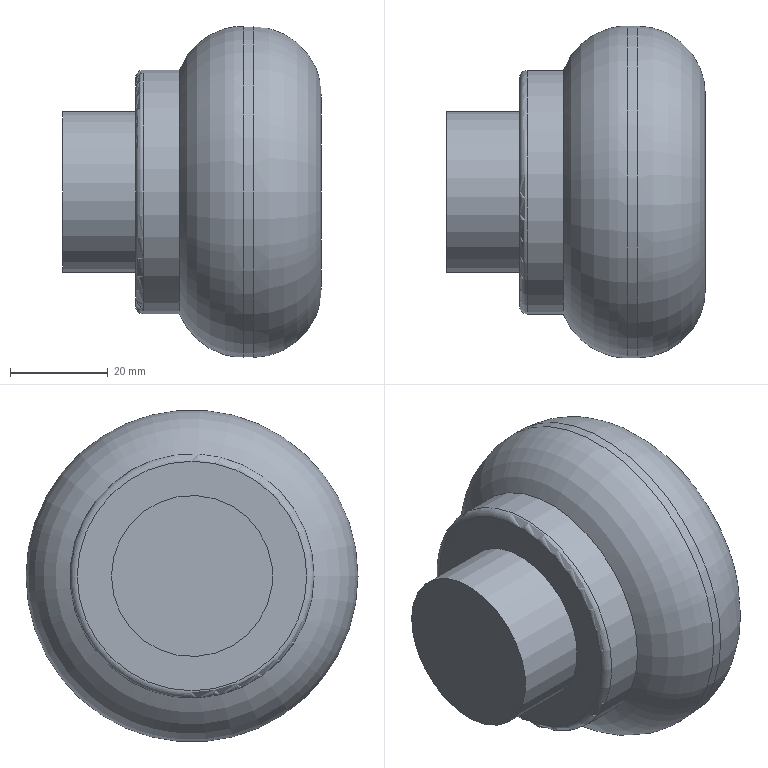Part | STEP file | CMT7E v7 | 1 solid | 11 faces | box 53 x 68 x 68 mm | volume 121265 mm3 | plane 4 | cylinder 4 | torus 3 | commonest cylinder face diameters 6 x1 33 x1 50 x1 68 x1
STEP:
#1=CARTESIAN_POINT('',(0.,0.,0.));
#2=DIRECTION('',(0.,0.,1.));
#3=DIRECTION('',(1.,0.,0.));
#4=AXIS2_PLACEMENT_3D('',#1,#2,#3);
#5=CARTESIAN_POINT('',(95.,16.49,190.));
#6=VERTEX_POINT('',#5);
#7=CARTESIAN_POINT('',(95.,-0.01,190.));
#8=DIRECTION('',(1.,0.,0.));
#9=DIRECTION('',(0.,1.,0.));
#10=AXIS2_PLACEMENT_3D('',#7,#8,#9);
#11=CIRCLE('',#10,16.5);
#12=CARTESIAN_POINT('',(95.,-0.01,190.));
#13=DIRECTION('',(1.,0.,0.));
#14=DIRECTION('',(0.,1.,0.));
#15=AXIS2_PLACEMENT_3D('',#12,#13,#14);
#16=PLANE('',#15);
#17=CARTESIAN_POINT('',(0.,0.));
#18=DIRECTION('',(1.,0.));
#19=AXIS2_PLACEMENT_2D('',#17,#18);
#20=CIRCLE('',#19,16.5);
#21=(GEOMETRIC_REPRESENTATION_CONTEXT(2)PARAMETRIC_REPRESENTATION_CONTEXT()REPRESENTATION_CONTEXT('',''));
#22=DEFINITIONAL_REPRESENTATION('',(#20),#21);
#23=PCURVE('',#16,#22);
#24=CARTESIAN_POINT('',(95.,-0.01,190.));
#25=DIRECTION('',(1.,0.,0.));
#26=DIRECTION('',(0.,1.,0.));
#27=AXIS2_PLACEMENT_3D('',#24,#25,#26);
#28=CYLINDRICAL_SURFACE('',#27,16.5);
#29=CARTESIAN_POINT('',(0.,0.));
#30=DIRECTION('',(1.,0.));
#31=VECTOR('',#30,1.);
#32=LINE('',#29,#31);
#33=(GEOMETRIC_REPRESENTATION_CONTEXT(2)PARAMETRIC_REPRESENTATION_CONTEXT()REPRESENTATION_CONTEXT('',''));
#34=DEFINITIONAL_REPRESENTATION('',(#32),#33);
#35=PCURVE('',#28,#34);
#36=SURFACE_CURVE('',#11,(#23,#35),.PCURVE_S1.);
#37=EDGE_CURVE('',#6,#6,#36,.T.);
#38=ORIENTED_EDGE('',*,*,#37,.F.);
#39=EDGE_LOOP('',(#38));
#40=FACE_BOUND('',#39,.T.);
#41=ADVANCED_FACE('',(#40),#16,.F.);
#42=ORIENTED_EDGE('',*,*,#37,.T.);
#43=CARTESIAN_POINT('',(110.,16.49,190.));
#44=VERTEX_POINT('',#43);
#45=CARTESIAN_POINT('',(95.,16.49,190.));
#46=CARTESIAN_POINT('',(110.,16.49,190.));
#47=B_SPLINE_CURVE_WITH_KNOTS('',1,(#45,#46),.UNSPECIFIED.,.F.,.F.,(2,2),(0.,15.),.PIECEWISE_BEZIER_KNOTS.);
#48=CARTESIAN_POINT('',(6.283,0.));
#49=DIRECTION('',(0.,1.));
#50=VECTOR('',#49,1.);
#51=LINE('',#48,#50);
#52=(GEOMETRIC_REPRESENTATION_CONTEXT(2)PARAMETRIC_REPRESENTATION_CONTEXT()REPRESENTATION_CONTEXT('',''));
#53=DEFINITIONAL_REPRESENTATION('',(#51),#52);
#54=PCURVE('',#28,#53);
#55=CARTESIAN_POINT('',(0.,0.));
#56=DIRECTION('',(0.,1.));
#57=VECTOR('',#56,1.);
#58=LINE('',#55,#57);
#59=(GEOMETRIC_REPRESENTATION_CONTEXT(2)PARAMETRIC_REPRESENTATION_CONTEXT()REPRESENTATION_CONTEXT('',''));
#60=DEFINITIONAL_REPRESENTATION('',(#58),#59);
#61=PCURVE('',#28,#60);
#62=SEAM_CURVE('',#47,(#54,#61),.PCURVE_S1.);
#63=EDGE_CURVE('',#6,#44,#62,.T.);
#64=ORIENTED_EDGE('',*,*,#63,.T.);
#65=CARTESIAN_POINT('',(110.,-0.01,190.));
#66=DIRECTION('',(-1.,0.,0.));
#67=DIRECTION('',(0.,1.,0.));
#68=AXIS2_PLACEMENT_3D('',#65,#66,#67);
#69=CIRCLE('',#68,16.5);
#70=CARTESIAN_POINT('',(6.283,15.));
#71=DIRECTION('',(-1.,0.));
#72=VECTOR('',#71,1.);
#73=LINE('',#70,#72);
#74=(GEOMETRIC_REPRESENTATION_CONTEXT(2)PARAMETRIC_REPRESENTATION_CONTEXT()REPRESENTATION_CONTEXT('',''));
#75=DEFINITIONAL_REPRESENTATION('',(#73),#74);
#76=PCURVE('',#28,#75);
#77=CARTESIAN_POINT('',(110.,-0.01,190.));
#78=DIRECTION('',(-1.,0.,0.));
#79=DIRECTION('',(0.,-1.,0.));
#80=AXIS2_PLACEMENT_3D('',#77,#78,#79);
#81=PLANE('',#80);
#82=CARTESIAN_POINT('',(0.,0.));
#83=DIRECTION('',(-1.,0.));
#84=AXIS2_PLACEMENT_2D('',#82,#83);
#85=CIRCLE('',#84,16.5);
#86=(GEOMETRIC_REPRESENTATION_CONTEXT(2)PARAMETRIC_REPRESENTATION_CONTEXT()REPRESENTATION_CONTEXT('',''));
#87=DEFINITIONAL_REPRESENTATION('',(#85),#86);
#88=PCURVE('',#81,#87);
#89=SURFACE_CURVE('',#69,(#76,#88),.PCURVE_S1.);
#90=EDGE_CURVE('',#44,#44,#89,.T.);
#91=ORIENTED_EDGE('',*,*,#90,.T.);
#92=ORIENTED_EDGE('',*,*,#63,.F.);
#93=EDGE_LOOP('',(#42,#64,#91,#92));
#94=FACE_BOUND('',#93,.T.);
#95=ADVANCED_FACE('',(#94),#28,.T.);
#96=CARTESIAN_POINT('',(148.,2.99,190.));
#97=VERTEX_POINT('',#96);
#98=CARTESIAN_POINT('',(148.,-0.01,190.));
#99=DIRECTION('',(-1.,0.,0.));
#100=DIRECTION('',(0.,1.,0.));
#101=AXIS2_PLACEMENT_3D('',#98,#99,#100);
#102=CIRCLE('',#101,3.);
#103=CARTESIAN_POINT('',(148.,-0.01,190.));
#104=DIRECTION('',(1.,0.,0.));
#105=DIRECTION('',(0.,1.,0.));
#106=AXIS2_PLACEMENT_3D('',#103,#104,#105);
#107=PLANE('',#106);
#108=CARTESIAN_POINT('',(3.,0.));
#109=CARTESIAN_POINT('',(3.,-5.196));
#110=CARTESIAN_POINT('',(-1.5,-2.598));
#111=CARTESIAN_POINT('',(-6.,0.));
#112=CARTESIAN_POINT('',(-1.5,2.598));
#113=CARTESIAN_POINT('',(3.,5.196));
#114=CARTESIAN_POINT('',(3.,0.));
#115=(BOUNDED_CURVE()B_SPLINE_CURVE(2,(#108,#109,#110,#111,#112,#113,#114),.UNSPECIFIED.,.T.,.F.)B_SPLINE_CURVE_WITH_KNOTS((1,2,2,2,2,1),(-2.094,0.,2.094,4.189,6.283,8.378),.UNSPECIFIED.)CURVE()GEOMETRIC_REPRESENTATION_ITEM()RATIONAL_B_SPLINE_CURVE((1.,0.5,1.,0.5,1.,0.5,1.))REPRESENTATION_ITEM(''));
#116=(GEOMETRIC_REPRESENTATION_CONTEXT(2)PARAMETRIC_REPRESENTATION_CONTEXT()REPRESENTATION_CONTEXT('',''));
#117=DEFINITIONAL_REPRESENTATION('',(#115),#116);
#118=PCURVE('',#107,#117);
#119=CARTESIAN_POINT('',(148.,-0.01,190.));
#120=DIRECTION('',(-1.,0.,0.));
#121=DIRECTION('',(0.,1.,0.));
#122=AXIS2_PLACEMENT_3D('',#119,#120,#121);
#123=CYLINDRICAL_SURFACE('',#122,3.);
#124=CARTESIAN_POINT('',(0.,0.));
#125=DIRECTION('',(1.,0.));
#126=VECTOR('',#125,1.);
#127=LINE('',#124,#126);
#128=(GEOMETRIC_REPRESENTATION_CONTEXT(2)PARAMETRIC_REPRESENTATION_CONTEXT()REPRESENTATION_CONTEXT('',''));
#129=DEFINITIONAL_REPRESENTATION('',(#127),#128);
#130=PCURVE('',#123,#129);
#131=SURFACE_CURVE('',#102,(#118,#130),.PCURVE_S1.);
#132=EDGE_CURVE('',#97,#97,#131,.T.);
#133=ORIENTED_EDGE('',*,*,#132,.T.);
#134=EDGE_LOOP('',(#133));
#135=FACE_BOUND('',#134,.T.);
#136=CARTESIAN_POINT('',(148.,19.99,190.));
#137=VERTEX_POINT('',#136);
#138=CARTESIAN_POINT('',(148.,-0.01,190.));
#139=DIRECTION('',(-1.,0.,0.));
#140=DIRECTION('',(0.,1.,0.));
#141=AXIS2_PLACEMENT_3D('',#138,#139,#140);
#142=CIRCLE('',#141,20.);
#143=CARTESIAN_POINT('',(20.,0.));
#144=CARTESIAN_POINT('',(20.,-34.641));
#145=CARTESIAN_POINT('',(-10.,-17.321));
#146=CARTESIAN_POINT('',(-40.,0.));
#147=CARTESIAN_POINT('',(-10.,17.321));
#148=CARTESIAN_POINT('',(20.,34.641));
#149=CARTESIAN_POINT('',(20.,0.));
#150=(BOUNDED_CURVE()B_SPLINE_CURVE(2,(#143,#144,#145,#146,#147,#148,#149),.UNSPECIFIED.,.T.,.F.)B_SPLINE_CURVE_WITH_KNOTS((1,2,2,2,2,1),(-2.094,0.,2.094,4.189,6.283,8.378),.UNSPECIFIED.)CURVE()GEOMETRIC_REPRESENTATION_ITEM()RATIONAL_B_SPLINE_CURVE((1.,0.5,1.,0.5,1.,0.5,1.))REPRESENTATION_ITEM(''));
#151=(GEOMETRIC_REPRESENTATION_CONTEXT(2)PARAMETRIC_REPRESENTATION_CONTEXT()REPRESENTATION_CONTEXT('',''));
#152=DEFINITIONAL_REPRESENTATION('',(#150),#151);
#153=PCURVE('',#107,#152);
#154=CARTESIAN_POINT('',(134.,-0.01,190.));
#155=DIRECTION('',(1.,0.,0.));
#156=DIRECTION('',(0.,0.,-1.));
#157=AXIS2_PLACEMENT_3D('',#154,#155,#156);
#158=TOROIDAL_SURFACE('',#157,20.,14.);
#159=CARTESIAN_POINT('',(7.854,1.571));
#160=DIRECTION('',(-1.,0.));
#161=VECTOR('',#160,1.);
#162=LINE('',#159,#161);
#163=(GEOMETRIC_REPRESENTATION_CONTEXT(2)PARAMETRIC_REPRESENTATION_CONTEXT()REPRESENTATION_CONTEXT('',''));
#164=DEFINITIONAL_REPRESENTATION('',(#162),#163);
#165=PCURVE('',#158,#164);
#166=SURFACE_CURVE('',#142,(#153,#165),.PCURVE_S1.);
#167=EDGE_CURVE('',#137,#137,#166,.T.);
#168=ORIENTED_EDGE('',*,*,#167,.F.);
#169=EDGE_LOOP('',(#168));
#170=FACE_BOUND('',#169,.T.);
#171=ADVANCED_FACE('',(#135,#170),#107,.T.);
#172=CARTESIAN_POINT('',(134.,33.99,190.));
#173=VERTEX_POINT('',#172);
#174=CARTESIAN_POINT('',(134.,-0.01,190.));
#175=DIRECTION('',(1.,0.,0.));
#176=DIRECTION('',(0.,1.,0.));
#177=AXIS2_PLACEMENT_3D('',#174,#175,#176);
#178=CIRCLE('',#177,34.);
#179=CARTESIAN_POINT('',(1.571,0.));
#180=DIRECTION('',(1.,0.));
#181=VECTOR('',#180,1.);
#182=LINE('',#179,#181);
#183=(GEOMETRIC_REPRESENTATION_CONTEXT(2)PARAMETRIC_REPRESENTATION_CONTEXT()REPRESENTATION_CONTEXT('',''));
#184=DEFINITIONAL_REPRESENTATION('',(#182),#183);
#185=PCURVE('',#158,#184);
#186=CARTESIAN_POINT('',(118.,-0.01,190.));
#187=DIRECTION('',(1.,0.,0.));
#188=DIRECTION('',(0.,1.,0.));
#189=AXIS2_PLACEMENT_3D('',#186,#187,#188);
#190=CYLINDRICAL_SURFACE('',#189,34.);
#191=CARTESIAN_POINT('',(0.,16.));
#192=DIRECTION('',(1.,0.));
#193=VECTOR('',#192,1.);
#194=LINE('',#191,#193);
#195=(GEOMETRIC_REPRESENTATION_CONTEXT(2)PARAMETRIC_REPRESENTATION_CONTEXT()REPRESENTATION_CONTEXT('',''));
#196=DEFINITIONAL_REPRESENTATION('',(#194),#195);
#197=PCURVE('',#190,#196);
#198=SURFACE_CURVE('',#178,(#185,#197),.PCURVE_S1.);
#199=EDGE_CURVE('',#173,#173,#198,.T.);
#200=ORIENTED_EDGE('',*,*,#199,.T.);
#201=CARTESIAN_POINT('',(134.,33.99,190.));
#202=CARTESIAN_POINT('',(137.743,33.99,190.));
#203=CARTESIAN_POINT('',(141.388,32.8,190.));
#204=CARTESIAN_POINT('',(144.527,30.517,190.));
#205=CARTESIAN_POINT('',(146.81,27.378,190.));
#206=CARTESIAN_POINT('',(148.,23.733,190.));
#207=CARTESIAN_POINT('',(148.,19.99,190.));
#208=(BOUNDED_CURVE()B_SPLINE_CURVE(6,(#201,#202,#203,#204,#205,#206,#207),.UNSPECIFIED.,.F.,.F.)B_SPLINE_CURVE_WITH_KNOTS((7,7),(0.,1.571),.PIECEWISE_BEZIER_KNOTS.)CURVE()GEOMETRIC_REPRESENTATION_ITEM()RATIONAL_B_SPLINE_CURVE((1.031,1.01,0.9979,0.994,0.9979,1.01,1.031))REPRESENTATION_ITEM(''));
#209=CARTESIAN_POINT('',(7.854,0.));
#210=DIRECTION('',(0.,1.));
#211=VECTOR('',#210,1.);
#212=LINE('',#209,#211);
#213=(GEOMETRIC_REPRESENTATION_CONTEXT(2)PARAMETRIC_REPRESENTATION_CONTEXT()REPRESENTATION_CONTEXT('',''));
#214=DEFINITIONAL_REPRESENTATION('',(#212),#213);
#215=PCURVE('',#158,#214);
#216=CARTESIAN_POINT('',(1.571,0.));
#217=DIRECTION('',(0.,1.));
#218=VECTOR('',#217,1.);
#219=LINE('',#216,#218);
#220=(GEOMETRIC_REPRESENTATION_CONTEXT(2)PARAMETRIC_REPRESENTATION_CONTEXT()REPRESENTATION_CONTEXT('',''));
#221=DEFINITIONAL_REPRESENTATION('',(#219),#220);
#222=PCURVE('',#158,#221);
#223=SEAM_CURVE('',#208,(#215,#222),.PCURVE_S1.);
#224=EDGE_CURVE('',#173,#137,#223,.T.);
#225=ORIENTED_EDGE('',*,*,#224,.T.);
#226=ORIENTED_EDGE('',*,*,#167,.T.);
#227=ORIENTED_EDGE('',*,*,#224,.F.);
#228=EDGE_LOOP('',(#200,#225,#226,#227));
#229=FACE_BOUND('',#228,.T.);
#230=ADVANCED_FACE('',(#229),#158,.T.);
#231=CARTESIAN_POINT('',(132.,33.99,190.));
#232=VERTEX_POINT('',#231);
#233=CARTESIAN_POINT('',(132.,-34.01,190.));
#234=VERTEX_POINT('',#233);
#235=CARTESIAN_POINT('',(132.,-0.01,190.));
#236=DIRECTION('',(-1.,0.,0.));
#237=DIRECTION('',(0.,1.,0.));
#238=AXIS2_PLACEMENT_3D('',#235,#236,#237);
#239=CIRCLE('',#238,34.);
#240=CARTESIAN_POINT('',(6.283,14.));
#241=DIRECTION('',(-1.,0.));
#242=VECTOR('',#241,1.);
#243=LINE('',#240,#242);
#244=(GEOMETRIC_REPRESENTATION_CONTEXT(2)PARAMETRIC_REPRESENTATION_CONTEXT()REPRESENTATION_CONTEXT('',''));
#245=DEFINITIONAL_REPRESENTATION('',(#243),#244);
#246=PCURVE('',#190,#245);
#247=CARTESIAN_POINT('',(132.,-0.01,190.));
#248=DIRECTION('',(1.,0.,0.));
#249=DIRECTION('',(0.,0.,-1.));
#250=AXIS2_PLACEMENT_3D('',#247,#248,#249);
#251=TOROIDAL_SURFACE('',#250,20.,14.);
#252=CARTESIAN_POINT('',(1.571,6.283));
#253=DIRECTION('',(-1.,0.));
#254=VECTOR('',#253,1.);
#255=LINE('',#252,#254);
#256=(GEOMETRIC_REPRESENTATION_CONTEXT(2)PARAMETRIC_REPRESENTATION_CONTEXT()REPRESENTATION_CONTEXT('',''));
#257=DEFINITIONAL_REPRESENTATION('',(#255),#256);
#258=PCURVE('',#251,#257);
#259=SURFACE_CURVE('',#239,(#246,#258),.PCURVE_S1.);
#260=EDGE_CURVE('',#232,#234,#259,.T.);
#261=ORIENTED_EDGE('',*,*,#260,.F.);
#262=CARTESIAN_POINT('',(132.,33.99,190.));
#263=CARTESIAN_POINT('',(134.,33.99,190.));
#264=B_SPLINE_CURVE_WITH_KNOTS('',1,(#262,#263),.UNSPECIFIED.,.F.,.F.,(2,2),(14.,16.),.PIECEWISE_BEZIER_KNOTS.);
#265=CARTESIAN_POINT('',(6.283,0.));
#266=DIRECTION('',(0.,1.));
#267=VECTOR('',#266,1.);
#268=LINE('',#265,#267);
#269=(GEOMETRIC_REPRESENTATION_CONTEXT(2)PARAMETRIC_REPRESENTATION_CONTEXT()REPRESENTATION_CONTEXT('',''));
#270=DEFINITIONAL_REPRESENTATION('',(#268),#269);
#271=PCURVE('',#190,#270);
#272=CARTESIAN_POINT('',(0.,0.));
#273=DIRECTION('',(0.,1.));
#274=VECTOR('',#273,1.);
#275=LINE('',#272,#274);
#276=(GEOMETRIC_REPRESENTATION_CONTEXT(2)PARAMETRIC_REPRESENTATION_CONTEXT()REPRESENTATION_CONTEXT('',''));
#277=DEFINITIONAL_REPRESENTATION('',(#275),#276);
#278=PCURVE('',#190,#277);
#279=SEAM_CURVE('',#264,(#271,#278),.PCURVE_S1.);
#280=EDGE_CURVE('',#232,#173,#279,.T.);
#281=ORIENTED_EDGE('',*,*,#280,.T.);
#282=ORIENTED_EDGE('',*,*,#199,.F.);
#283=ORIENTED_EDGE('',*,*,#280,.F.);
#284=CARTESIAN_POINT('',(132.,-0.01,190.));
#285=DIRECTION('',(-1.,0.,0.));
#286=DIRECTION('',(0.,1.,0.));
#287=AXIS2_PLACEMENT_3D('',#284,#285,#286);
#288=CIRCLE('',#287,34.);
#289=CARTESIAN_POINT('',(6.283,14.));
#290=DIRECTION('',(-1.,0.));
#291=VECTOR('',#290,1.);
#292=LINE('',#289,#291);
#293=(GEOMETRIC_REPRESENTATION_CONTEXT(2)PARAMETRIC_REPRESENTATION_CONTEXT()REPRESENTATION_CONTEXT('',''));
#294=DEFINITIONAL_REPRESENTATION('',(#292),#293);
#295=PCURVE('',#190,#294);
#296=CARTESIAN_POINT('',(7.854,6.283));
#297=DIRECTION('',(-1.,0.));
#298=VECTOR('',#297,1.);
#299=LINE('',#296,#298);
#300=(GEOMETRIC_REPRESENTATION_CONTEXT(2)PARAMETRIC_REPRESENTATION_CONTEXT()REPRESENTATION_CONTEXT('',''));
#301=DEFINITIONAL_REPRESENTATION('',(#299),#300);
#302=PCURVE('',#251,#301);
#303=SURFACE_CURVE('',#288,(#295,#302),.PCURVE_S1.);
#304=EDGE_CURVE('',#234,#232,#303,.T.);
#305=ORIENTED_EDGE('',*,*,#304,.F.);
#306=EDGE_LOOP('',(#261,#281,#282,#283,#305));
#307=FACE_BOUND('',#306,.T.);
#308=ADVANCED_FACE('',(#307),#190,.T.);
#309=CARTESIAN_POINT('',(118.923,-25.01,190.));
#310=VERTEX_POINT('',#309);
#311=CARTESIAN_POINT('',(118.923,-0.01,190.));
#312=DIRECTION('',(1.,0.,0.));
#313=DIRECTION('',(0.,-1.,0.));
#314=AXIS2_PLACEMENT_3D('',#311,#312,#313);
#315=CIRCLE('',#314,25.);
#316=CARTESIAN_POINT('',(-1.571,5.078));
#317=DIRECTION('',(1.,0.));
#318=VECTOR('',#317,1.);
#319=LINE('',#316,#318);
#320=(GEOMETRIC_REPRESENTATION_CONTEXT(2)PARAMETRIC_REPRESENTATION_CONTEXT()REPRESENTATION_CONTEXT('',''));
#321=DEFINITIONAL_REPRESENTATION('',(#319),#320);
#322=PCURVE('',#251,#321);
#323=CARTESIAN_POINT('',(118.,-0.01,190.));
#324=DIRECTION('',(-1.,0.,0.));
#325=DIRECTION('',(0.,-1.,0.));
#326=AXIS2_PLACEMENT_3D('',#323,#324,#325);
#327=CYLINDRICAL_SURFACE('',#326,25.);
#328=CARTESIAN_POINT('',(6.283,-0.9233));
#329=DIRECTION('',(-1.,0.));
#330=VECTOR('',#329,1.);
#331=LINE('',#328,#330);
#332=(GEOMETRIC_REPRESENTATION_CONTEXT(2)PARAMETRIC_REPRESENTATION_CONTEXT()REPRESENTATION_CONTEXT('',''));
#333=DEFINITIONAL_REPRESENTATION('',(#331),#332);
#334=PCURVE('',#327,#333);
#335=SURFACE_CURVE('',#315,(#322,#334),.PCURVE_S1.);
#336=EDGE_CURVE('',#310,#310,#335,.T.);
#337=ORIENTED_EDGE('',*,*,#336,.T.);
#338=CARTESIAN_POINT('',(118.923,-25.01,190.));
#339=CARTESIAN_POINT('',(119.94,-27.67,190.));
#340=CARTESIAN_POINT('',(121.588,-30.043,190.));
#341=CARTESIAN_POINT('',(123.77,-31.968,190.));
#342=CARTESIAN_POINT('',(126.347,-33.318,190.));
#343=CARTESIAN_POINT('',(129.152,-34.01,190.));
#344=CARTESIAN_POINT('',(132.,-34.01,190.));
#345=(BOUNDED_CURVE()B_SPLINE_CURVE(6,(#338,#339,#340,#341,#342,#343,#344),.UNSPECIFIED.,.F.,.F.)B_SPLINE_CURVE_WITH_KNOTS((7,7),(5.078,6.283),.PIECEWISE_BEZIER_KNOTS.)CURVE()GEOMETRIC_REPRESENTATION_ITEM()RATIONAL_B_SPLINE_CURVE((1.018,1.006,0.9988,0.9964,0.9988,1.006,1.018))REPRESENTATION_ITEM(''));
#346=CARTESIAN_POINT('',(4.712,0.));
#347=DIRECTION('',(0.,1.));
#348=VECTOR('',#347,1.);
#349=LINE('',#346,#348);
#350=(GEOMETRIC_REPRESENTATION_CONTEXT(2)PARAMETRIC_REPRESENTATION_CONTEXT()REPRESENTATION_CONTEXT('',''));
#351=DEFINITIONAL_REPRESENTATION('',(#349),#350);
#352=PCURVE('',#251,#351);
#353=CARTESIAN_POINT('',(-1.571,0.));
#354=DIRECTION('',(0.,1.));
#355=VECTOR('',#354,1.);
#356=LINE('',#353,#355);
#357=(GEOMETRIC_REPRESENTATION_CONTEXT(2)PARAMETRIC_REPRESENTATION_CONTEXT()REPRESENTATION_CONTEXT('',''));
#358=DEFINITIONAL_REPRESENTATION('',(#356),#357);
#359=PCURVE('',#251,#358);
#360=SEAM_CURVE('',#345,(#352,#359),.PCURVE_S1.);
#361=EDGE_CURVE('',#310,#234,#360,.T.);
#362=ORIENTED_EDGE('',*,*,#361,.T.);
#363=ORIENTED_EDGE('',*,*,#304,.T.);
#364=ORIENTED_EDGE('',*,*,#260,.T.);
#365=ORIENTED_EDGE('',*,*,#361,.F.);
#366=EDGE_LOOP('',(#337,#362,#363,#364,#365));
#367=FACE_BOUND('',#366,.T.);
#368=ADVANCED_FACE('',(#367),#251,.T.);
#369=CARTESIAN_POINT('',(146.,2.99,190.));
#370=VERTEX_POINT('',#369);
#371=CARTESIAN_POINT('',(146.,-0.01,190.));
#372=DIRECTION('',(-1.,0.,0.));
#373=DIRECTION('',(0.,1.,0.));
#374=AXIS2_PLACEMENT_3D('',#371,#372,#373);
#375=CIRCLE('',#374,3.);
#376=CARTESIAN_POINT('',(146.,-0.01,190.));
#377=DIRECTION('',(1.,0.,0.));
#378=DIRECTION('',(0.,1.,0.));
#379=AXIS2_PLACEMENT_3D('',#376,#377,#378);
#380=PLANE('',#379);
#381=CARTESIAN_POINT('',(3.,0.));
#382=CARTESIAN_POINT('',(3.,-5.196));
#383=CARTESIAN_POINT('',(-1.5,-2.598));
#384=CARTESIAN_POINT('',(-6.,0.));
#385=CARTESIAN_POINT('',(-1.5,2.598));
#386=CARTESIAN_POINT('',(3.,5.196));
#387=CARTESIAN_POINT('',(3.,0.));
#388=(BOUNDED_CURVE()B_SPLINE_CURVE(2,(#381,#382,#383,#384,#385,#386,#387),.UNSPECIFIED.,.T.,.F.)B_SPLINE_CURVE_WITH_KNOTS((1,2,2,2,2,1),(-2.094,0.,2.094,4.189,6.283,8.378),.UNSPECIFIED.)CURVE()GEOMETRIC_REPRESENTATION_ITEM()RATIONAL_B_SPLINE_CURVE((1.,0.5,1.,0.5,1.,0.5,1.))REPRESENTATION_ITEM(''));
#389=(GEOMETRIC_REPRESENTATION_CONTEXT(2)PARAMETRIC_REPRESENTATION_CONTEXT()REPRESENTATION_CONTEXT('',''));
#390=DEFINITIONAL_REPRESENTATION('',(#388),#389);
#391=PCURVE('',#380,#390);
#392=CARTESIAN_POINT('',(0.,2.));
#393=DIRECTION('',(1.,0.));
#394=VECTOR('',#393,1.);
#395=LINE('',#392,#394);
#396=(GEOMETRIC_REPRESENTATION_CONTEXT(2)PARAMETRIC_REPRESENTATION_CONTEXT()REPRESENTATION_CONTEXT('',''));
#397=DEFINITIONAL_REPRESENTATION('',(#395),#396);
#398=PCURVE('',#123,#397);
#399=SURFACE_CURVE('',#375,(#391,#398),.PCURVE_S1.);
#400=EDGE_CURVE('',#370,#370,#399,.T.);
#401=ORIENTED_EDGE('',*,*,#400,.F.);
#402=EDGE_LOOP('',(#401));
#403=FACE_BOUND('',#402,.T.);
#404=ADVANCED_FACE('',(#403),#380,.T.);
#405=ORIENTED_EDGE('',*,*,#400,.F.);
#406=CARTESIAN_POINT('',(148.,2.99,190.));
#407=CARTESIAN_POINT('',(146.,2.99,190.));
#408=B_SPLINE_CURVE_WITH_KNOTS('',1,(#406,#407),.UNSPECIFIED.,.F.,.F.,(2,2),(0.,2.),.PIECEWISE_BEZIER_KNOTS.);
#409=CARTESIAN_POINT('',(0.,0.));
#410=DIRECTION('',(0.,1.));
#411=VECTOR('',#410,1.);
#412=LINE('',#409,#411);
#413=(GEOMETRIC_REPRESENTATION_CONTEXT(2)PARAMETRIC_REPRESENTATION_CONTEXT()REPRESENTATION_CONTEXT('',''));
#414=DEFINITIONAL_REPRESENTATION('',(#412),#413);
#415=PCURVE('',#123,#414);
#416=CARTESIAN_POINT('',(6.283,0.));
#417=DIRECTION('',(0.,1.));
#418=VECTOR('',#417,1.);
#419=LINE('',#416,#418);
#420=(GEOMETRIC_REPRESENTATION_CONTEXT(2)PARAMETRIC_REPRESENTATION_CONTEXT()REPRESENTATION_CONTEXT('',''));
#421=DEFINITIONAL_REPRESENTATION('',(#419),#420);
#422=PCURVE('',#123,#421);
#423=SEAM_CURVE('',#408,(#415,#422),.PCURVE_S1.);
#424=EDGE_CURVE('',#97,#370,#423,.T.);
#425=ORIENTED_EDGE('',*,*,#424,.F.);
#426=ORIENTED_EDGE('',*,*,#132,.T.);
#427=ORIENTED_EDGE('',*,*,#424,.T.);
#428=EDGE_LOOP('',(#405,#425,#426,#427));
#429=FACE_BOUND('',#428,.F.);
#430=ADVANCED_FACE('',(#429),#123,.F.);
#431=ORIENTED_EDGE('',*,*,#90,.F.);
#432=EDGE_LOOP('',(#431));
#433=FACE_BOUND('',#432,.T.);
#434=CARTESIAN_POINT('',(110.,-23.51,190.));
#435=VERTEX_POINT('',#434);
#436=CARTESIAN_POINT('',(110.,-0.01,190.));
#437=DIRECTION('',(1.,0.,0.));
#438=DIRECTION('',(0.,-1.,0.));
#439=AXIS2_PLACEMENT_3D('',#436,#437,#438);
#440=CIRCLE('',#439,23.5);
#441=CARTESIAN_POINT('',(23.5,0.));
#442=CARTESIAN_POINT('',(23.5,-40.703));
#443=CARTESIAN_POINT('',(-11.75,-20.352));
#444=CARTESIAN_POINT('',(-47.,0.));
#445=CARTESIAN_POINT('',(-11.75,20.352));
#446=CARTESIAN_POINT('',(23.5,40.703));
#447=CARTESIAN_POINT('',(23.5,0.));
#448=(BOUNDED_CURVE()B_SPLINE_CURVE(2,(#441,#442,#443,#444,#445,#446,#447),.UNSPECIFIED.,.T.,.F.)B_SPLINE_CURVE_WITH_KNOTS((1,2,2,2,2,1),(-2.094,0.,2.094,4.189,6.283,8.378),.UNSPECIFIED.)CURVE()GEOMETRIC_REPRESENTATION_ITEM()RATIONAL_B_SPLINE_CURVE((1.,0.5,1.,0.5,1.,0.5,1.))REPRESENTATION_ITEM(''));
#449=(GEOMETRIC_REPRESENTATION_CONTEXT(2)PARAMETRIC_REPRESENTATION_CONTEXT()REPRESENTATION_CONTEXT('',''));
#450=DEFINITIONAL_REPRESENTATION('',(#448),#449);
#451=PCURVE('',#81,#450);
#452=CARTESIAN_POINT('',(111.5,-0.01,190.));
#453=DIRECTION('',(-1.,0.,0.));
#454=DIRECTION('',(0.,0.,1.));
#455=AXIS2_PLACEMENT_3D('',#452,#453,#454);
#456=TOROIDAL_SURFACE('',#455,23.5,1.5);
#457=CARTESIAN_POINT('',(4.712,1.571));
#458=DIRECTION('',(-1.,0.));
#459=VECTOR('',#458,1.);
#460=LINE('',#457,#459);
#461=(GEOMETRIC_REPRESENTATION_CONTEXT(2)PARAMETRIC_REPRESENTATION_CONTEXT()REPRESENTATION_CONTEXT('',''));
#462=DEFINITIONAL_REPRESENTATION('',(#460),#461);
#463=PCURVE('',#456,#462);
#464=SURFACE_CURVE('',#440,(#451,#463),.PCURVE_S1.);
#465=EDGE_CURVE('',#435,#435,#464,.T.);
#466=ORIENTED_EDGE('',*,*,#465,.F.);
#467=EDGE_LOOP('',(#466));
#468=FACE_BOUND('',#467,.T.);
#469=ADVANCED_FACE('',(#433,#468),#81,.T.);
#470=ORIENTED_EDGE('',*,*,#336,.F.);
#471=CARTESIAN_POINT('',(111.5,-25.01,190.));
#472=VERTEX_POINT('',#471);
#473=CARTESIAN_POINT('',(118.923,-25.01,190.));
#474=CARTESIAN_POINT('',(111.5,-25.01,190.));
#475=B_SPLINE_CURVE_WITH_KNOTS('',1,(#473,#474),.UNSPECIFIED.,.F.,.F.,(2,2),(-0.9233,6.5),.PIECEWISE_BEZIER_KNOTS.);
#476=CARTESIAN_POINT('',(6.283,0.));
#477=DIRECTION('',(0.,1.));
#478=VECTOR('',#477,1.);
#479=LINE('',#476,#478);
#480=(GEOMETRIC_REPRESENTATION_CONTEXT(2)PARAMETRIC_REPRESENTATION_CONTEXT()REPRESENTATION_CONTEXT('',''));
#481=DEFINITIONAL_REPRESENTATION('',(#479),#480);
#482=PCURVE('',#327,#481);
#483=CARTESIAN_POINT('',(0.,0.));
#484=DIRECTION('',(0.,1.));
#485=VECTOR('',#484,1.);
#486=LINE('',#483,#485);
#487=(GEOMETRIC_REPRESENTATION_CONTEXT(2)PARAMETRIC_REPRESENTATION_CONTEXT()REPRESENTATION_CONTEXT('',''));
#488=DEFINITIONAL_REPRESENTATION('',(#486),#487);
#489=PCURVE('',#327,#488);
#490=SEAM_CURVE('',#475,(#482,#489),.PCURVE_S1.);
#491=EDGE_CURVE('',#310,#472,#490,.T.);
#492=ORIENTED_EDGE('',*,*,#491,.T.);
#493=CARTESIAN_POINT('',(111.5,-0.01,190.));
#494=DIRECTION('',(-1.,0.,0.));
#495=DIRECTION('',(0.,-1.,0.));
#496=AXIS2_PLACEMENT_3D('',#493,#494,#495);
#497=CIRCLE('',#496,25.);
#498=CARTESIAN_POINT('',(0.,6.5));
#499=DIRECTION('',(1.,0.));
#500=VECTOR('',#499,1.);
#501=LINE('',#498,#500);
#502=(GEOMETRIC_REPRESENTATION_CONTEXT(2)PARAMETRIC_REPRESENTATION_CONTEXT()REPRESENTATION_CONTEXT('',''));
#503=DEFINITIONAL_REPRESENTATION('',(#501),#502);
#504=PCURVE('',#327,#503);
#505=CARTESIAN_POINT('',(-1.571,0.));
#506=DIRECTION('',(1.,0.));
#507=VECTOR('',#506,1.);
#508=LINE('',#505,#507);
#509=(GEOMETRIC_REPRESENTATION_CONTEXT(2)PARAMETRIC_REPRESENTATION_CONTEXT()REPRESENTATION_CONTEXT('',''));
#510=DEFINITIONAL_REPRESENTATION('',(#508),#509);
#511=PCURVE('',#456,#510);
#512=SURFACE_CURVE('',#497,(#504,#511),.PCURVE_S1.);
#513=EDGE_CURVE('',#472,#472,#512,.T.);
#514=ORIENTED_EDGE('',*,*,#513,.F.);
#515=ORIENTED_EDGE('',*,*,#491,.F.);
#516=EDGE_LOOP('',(#470,#492,#514,#515));
#517=FACE_BOUND('',#516,.T.);
#518=ADVANCED_FACE('',(#517),#327,.T.);
#519=ORIENTED_EDGE('',*,*,#513,.T.);
#520=CARTESIAN_POINT('',(111.5,-25.01,190.));
#521=CARTESIAN_POINT('',(111.099,-25.01,190.));
#522=CARTESIAN_POINT('',(110.708,-24.882,190.));
#523=CARTESIAN_POINT('',(110.372,-24.638,190.));
#524=CARTESIAN_POINT('',(110.128,-24.302,190.));
#525=CARTESIAN_POINT('',(110.,-23.911,190.));
#526=CARTESIAN_POINT('',(110.,-23.51,190.));
#527=(BOUNDED_CURVE()B_SPLINE_CURVE(6,(#520,#521,#522,#523,#524,#525,#526),.UNSPECIFIED.,.F.,.F.)B_SPLINE_CURVE_WITH_KNOTS((7,7),(0.,1.571),.PIECEWISE_BEZIER_KNOTS.)CURVE()GEOMETRIC_REPRESENTATION_ITEM()RATIONAL_B_SPLINE_CURVE((1.031,1.01,0.9979,0.994,0.9979,1.01,1.031))REPRESENTATION_ITEM(''));
#528=CARTESIAN_POINT('',(4.712,0.));
#529=DIRECTION('',(0.,1.));
#530=VECTOR('',#529,1.);
#531=LINE('',#528,#530);
#532=(GEOMETRIC_REPRESENTATION_CONTEXT(2)PARAMETRIC_REPRESENTATION_CONTEXT()REPRESENTATION_CONTEXT('',''));
#533=DEFINITIONAL_REPRESENTATION('',(#531),#532);
#534=PCURVE('',#456,#533);
#535=CARTESIAN_POINT('',(-1.571,0.));
#536=DIRECTION('',(0.,1.));
#537=VECTOR('',#536,1.);
#538=LINE('',#535,#537);
#539=(GEOMETRIC_REPRESENTATION_CONTEXT(2)PARAMETRIC_REPRESENTATION_CONTEXT()REPRESENTATION_CONTEXT('',''));
#540=DEFINITIONAL_REPRESENTATION('',(#538),#539);
#541=PCURVE('',#456,#540);
#542=SEAM_CURVE('',#527,(#534,#541),.PCURVE_S1.);
#543=EDGE_CURVE('',#472,#435,#542,.T.);
#544=ORIENTED_EDGE('',*,*,#543,.T.);
#545=ORIENTED_EDGE('',*,*,#465,.T.);
#546=ORIENTED_EDGE('',*,*,#543,.F.);
#547=EDGE_LOOP('',(#519,#544,#545,#546));
#548=FACE_BOUND('',#547,.T.);
#549=ADVANCED_FACE('',(#548),#456,.T.);
#550=CLOSED_SHELL('',(#41,#95,#171,#230,#308,#368,#404,#430,#469,#518,#549));
#551=MANIFOLD_SOLID_BREP('',#550);
#552=(LENGTH_UNIT()NAMED_UNIT(*)SI_UNIT(.MILLI.,.METRE.));
#553=UNCERTAINTY_MEASURE_WITH_UNIT(LENGTH_MEASURE(0.0000005),#552,'','');
#554=(NAMED_UNIT(*)PLANE_ANGLE_UNIT()SI_UNIT($,.RADIAN.));
#555=(NAMED_UNIT(*)SI_UNIT($,.STERADIAN.)SOLID_ANGLE_UNIT());
#556=(GEOMETRIC_REPRESENTATION_CONTEXT(3)GLOBAL_UNCERTAINTY_ASSIGNED_CONTEXT((#553))GLOBAL_UNIT_ASSIGNED_CONTEXT((#552,#554,#555))REPRESENTATION_CONTEXT('',''));
#557=ADVANCED_BREP_SHAPE_REPRESENTATION('',(#4,#551),#556);